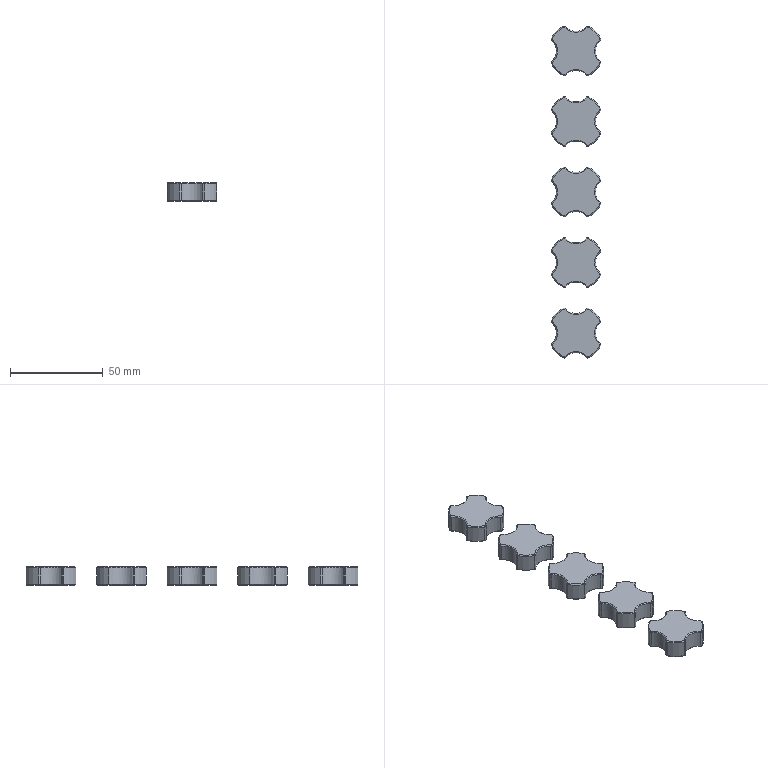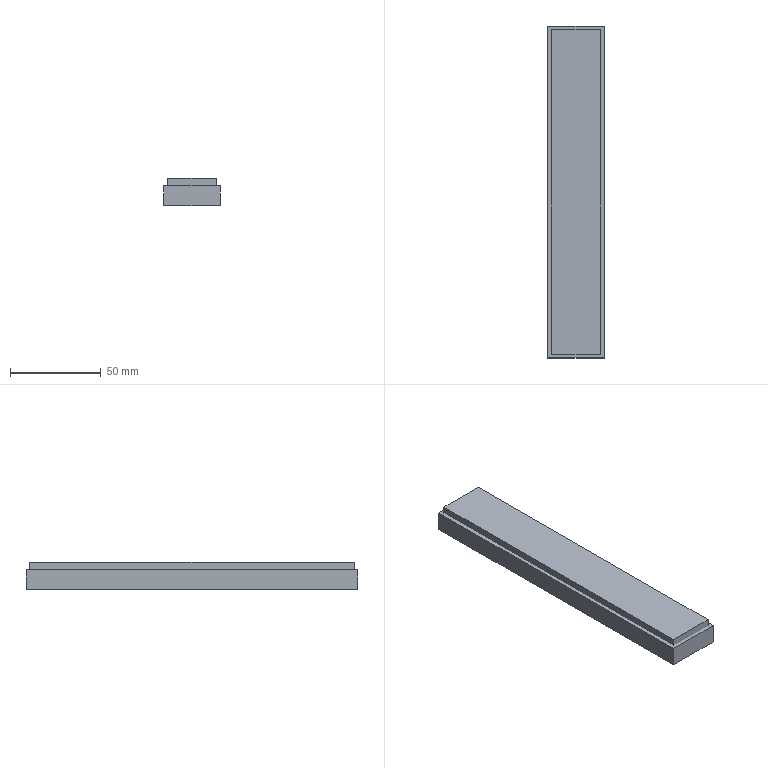CAM job | NX | 3-axis milling | part box 26.875 x 178.875 x 10 mm | stock box 30.875 x 182.875 x 15 mm
Tools:
number,name,description,diameter,corner_radius,flute_length,length,flutes
19,D80,Milling Tool-5 Parameters,80.0,0.0,50.0,75.0,2
15,D10,Milling Tool-5 Parameters,10.0,0.0,50.0,75.0,2
14,D10JING,Milling Tool-5 Parameters,10.0,0.0,50.0,75.0,2
17,D3,Milling Tool-5 Parameters,3.0,0.0,50.0,75.0,2
1,D6A45,Milling Tool-5 Parameters,6.0,0.0,50.0,75.0,2
Operations:
program,operation,operation_type,tool,method,geometry_group,spindle_rpm,surface_speed,feed_per_tooth,feed_cut,feed_plunge,cut_length_mm,path_length_mm,cut_time_min,machine_time_min
1,FLOOR_WALL,VolumeBased25DMillingOperation,D80,METHOD,A,6500.0,1633.0,0.1154,1500.0,100.0,278.875,332.875,0.1859,0.1913
1,ZLEVEL_PROFILE_COPY_1,ZLevelMilling,D10,METHOD,A,9500.0,298.0,0.1842,3500.0,1000.0,7459.079,8210.407,2.302,2.377
1,ZLEVEL_PROFILE_COPY_1_COPY,ZLevelMilling,D10JING,METHOD,A,9500.0,298.0,0.0632,1200.0,1000.0,678.211,1531.579,0.5673,0.6526
1,HOLE_MILLING,CylinderMilling,D3,METHOD,A,9500.0,89.0,0.0605,1150.0,100.0,397.701,882.201,0.3458,0.3943
1,PLANAR_MILL_COPY_COPY_COPY_COPY,PlanarMilling,D6A45,METHOD,A,9500.0,179.0,0.0658,1250.0,100.0,609.428,1447.229,0.4875,0.5713
1,刀补17,CylinderMilling,D3,METHOD,A,9500.0,89.0,0.0605,1150.0,100.0,86.067,570.567,0.0748,0.1233
2,FLOOR_WALL_COPY,VolumeBased25DMillingOperation,D80,METHOD,B,6500.0,1633.0,0.1154,1500.0,100.0,2748.75,5663.627,1.833,2.124
2,PLANAR_MILL_COPY_COPY_COPY_COPY_COPY,PlanarMilling,D6A45,METHOD,B,9500.0,179.0,0.0658,1250.0,100.0,552.54,976.368,0.442,0.4844